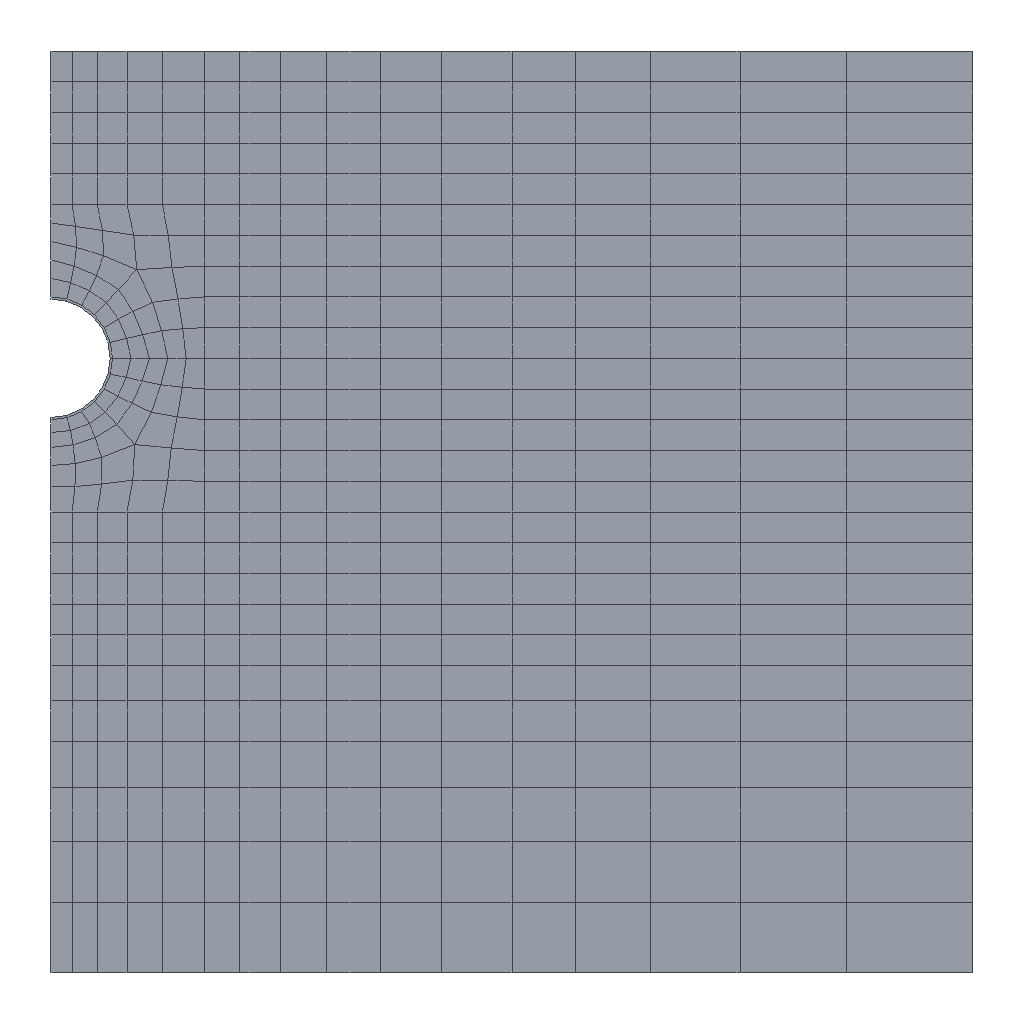Simulation study | abaqus
Set-up summary:
category,name,step,type,value,unit,region
solver,abaqus,,Abaqus/CAE 2024
units,mm-mN-s-kg (kPa) or mm-kg-s,,inferred,E=2e+07 density=
analysis,geo,,geostatic
analysis,relax-1,,static,time_period=1
analysis,add,,static,time_period=1
analysis,relax-2,,static,time_period=1
mesh,nodes,,,509
mesh,elements,,,446
element_type,CPE4,,,434
element_type,CPE4I,,,12
material,liner,,E,2e+07
material,liner,,nu,0.2
material,soil,,E,200000
material,soil,,nu,0.2
section,liner,,solid section,,,_PickedSet2
section,soil,,solid section,,,_PickedSet74
load,stress,initial,initial condition stress
load,Load-1,geo,by,-20,,_PickedSet6
load,,geo,concentrated force,"206.968 [dir=(0.9999, -0.0142, 0) n=2]",,soil-1.19
load,,geo,concentrated force,"273.813 [dir=(0.4268, -0.9043, 0) n=2]",,soil-1.20
load,,geo,concentrated force,"196.306 [dir=(0.5272, 0.8498, 0) n=2]",,soil-1.24
load,,geo,concentrated force,"239.406 [dir=(0.8773, -0.48, 0) n=2]",,soil-1.138
load,,geo,concentrated force,"301.488 [dir=(0.6514, -0.7587, 0) n=2]",,soil-1.139
load,,geo,concentrated force,"372.569 [dir=(0.445, -0.8955, 0) n=2]",,soil-1.140
load,,geo,concentrated force,"435.986 [dir=(0.2755, -0.9613, 0) n=2]",,soil-1.141
load,,geo,concentrated force,"479.559 [dir=(0.1318, -0.9913, 0) n=2]",,soil-1.142
load,,geo,concentrated force,"327.658 [dir=(0.1347, 0.9909, 0) n=2]",,soil-1.167
load,,geo,concentrated force,"310.398 [dir=(0.28, 0.96, 0) n=2]",,soil-1.168
load,,geo,concentrated force,"281.973 [dir=(0.4505, 0.8928, 0) n=2]",,soil-1.169
load,,geo,concentrated force,"246.244 [dir=(0.6591, 0.7521, 0) n=2]",,soil-1.170
load,,geo,concentrated force,"214.419 [dir=(0.8862, 0.4633, 0) n=2]",,soil-1.171
load,Load-2,relax-2,pressure,50,,_PickedSurf22
bc,BC-1,initial,fixed,[dofs=x],,_PickedSet12
bc,BC-2,initial,fixed,"[dofs=x,y n=2]",,_PickedSet13
bc,BC-3,initial,fixed,[dofs=x],,_PickedSet19
contact,Int-1,initial,contact pair surface to surface,interaction=IntProp-1; friction=0; behavior=hard,,tunnel / liner
Abaqus input file, long lists of numbers shortened:
*Heading
** Job name: deck Model name: Model-1
** Generated by: Abaqus/CAE 2024
*Preprint, echo=NO, model=NO, history=NO, contact=NO
**
** PARTS
**
*Part, name=Liner
*Node
      1,           0.,           4.
      2,           0.,    3.85
** (24 more lines like these left out)
*Element, type=CPE4I
 1,  1,  2,  4,  3
 2,  3,  4,  6,  5
** (10 more lines like these left out)
*Nset, nset=_PickedSet2, internal, generate
  1,  26,   1
*Elset, elset=_PickedSet2, internal, generate
  1,  12,   1
*Nset, nset=liner, generate
  1,  26,   1
*Elset, elset=liner, generate
  1,  12,   1
** Section: liner
*Solid Section, elset=_PickedSet2, material=liner
,
*End Part
**
*Part, name=soil
*Node
      1,          60.,         -10.
      2,          30.,         -10.
** (481 more lines like these left out)
*Element, type=CPE4
 1,   1,  27, 199,  42
 2,  27,  28, 200, 199
** (432 more lines like these left out)
*Nset, nset=all, generate
   1,  483,    1
*Elset, elset=all, generate
   1,  434,    1
*Nset, nset=_PickedSet74, internal, generate
   1,  483,    1
*Elset, elset=_PickedSet74, internal, generate
   1,  434,    1
*Nset, nset=tunnel
  19,  20,  24, 138, 139, 140, 141, 142, 167, 168, 169, 170, 171
*Elset, elset=tunnel
 214, 217, 220, 221, 222, 223, 292, 295, 298, 299, 300, 301
** Section: soil
*Solid Section, elset=_PickedSet74, material=soil
1.,
*End Part
**
**
** ASSEMBLY
**
*Assembly, name=Assembly
**
*Instance, name=soil-1, part=soil
*End Instance
**
*Instance, name=Liner-1, part=Liner
*End Instance
**
*Nset, nset=_PickedSet6, internal, instance=soil-1, generate
   1,  483,    1
*Elset, elset=_PickedSet6, internal, instance=soil-1, generate
   1,  434,    1
*Nset, nset=_PickedSet11, internal, instance=soil-1, generate
   1,  483,    1
*Elset, elset=_PickedSet11, internal, instance=soil-1, generate
   1,  434,    1
*Nset, nset=_PickedSet12, internal, instance=soil-1
   1,   4,   7,   8,  10,  11,  14,  20,  21,  22,  23,  24,  26,  39,  40,  41
  42,  52,  53,  54,  55,  56,  69,  70,  71,  72,  95,  96,  97,  98, 126, 127
** (2 more lines like these left out)
*Elset, elset=_PickedSet12, internal, instance=soil-1
   1,   6,  11,  16,  21,  50,  51,  52,  53,  54,  55,  76,  77,  78,  79,  80
 111, 116, 121, 126, 131, 196, 197, 223, 226, 229, 250, 251, 252, 253, 254, 259
** (2 more lines like these left out)
*Nset, nset=_PickedSet13, internal, instance=soil-1
   5,   8,  25,  26,  57,  58,  59,  60, 185, 186, 187, 188, 194, 195, 196, 197
 198,
*Elset, elset=_PickedSet13, internal, instance=soil-1
  26,  32,  38,  44,  50, 364, 365, 366, 367, 368, 404, 410, 416, 422, 428, 434
*Nset, nset=_PickedSet19, internal, instance=Liner-1
  1,  2, 25, 26
*Elset, elset=_PickedSet19, internal, instance=Liner-1
  1, 12
*Elset, elset=_liner_S4, internal, instance=Liner-1, generate
  1,  12,   1
*Surface, type=ELEMENT, name=liner
_liner_S4, S4
*Elset, elset=_tunnel_S2, internal, instance=soil-1
 214, 217, 220, 292, 295, 298
*Elset, elset=_tunnel_S1, internal, instance=soil-1
 221, 222, 223, 299, 300, 301
*Surface, type=ELEMENT, name=tunnel
_tunnel_S2, S2
_tunnel_S1, S1
*Elset, elset=__PickedSurf22_S4, internal, instance=soil-1, generate
 166,  191,    5
*Elset, elset=__PickedSurf22_S2, internal, instance=soil-1, generate
 234,  254,    5
*Surface, type=ELEMENT, name=_PickedSurf22, internal
__PickedSurf22_S4, S4
__PickedSurf22_S2, S2
*End Assembly
*Amplitude, name=Relax, time=TOTAL TIME
             0.,              1.,              1.,              1.,              2.,             0.6,              3.,             0.6
             4.,              0.
**
** MATERIALS
**
*Material, name=liner
*Elastic
 2e+07, 0.2
*Material, name=soil
*Elastic
200000., 0.2
**
** INTERACTION PROPERTIES
**
*Surface Interaction, name=IntProp-1
1.,
*Friction
0.,
*Surface Behavior, pressure-overclosure=HARD
**
** BOUNDARY CONDITIONS
**
** Name: BC-1 Type: Displacement/Rotation
*Boundary
_PickedSet12, 1, 1
** Name: BC-2 Type: Displacement/Rotation
*Boundary
_PickedSet13, 1, 1
_PickedSet13, 2, 2
** Name: BC-3 Type: Displacement/Rotation
*Boundary
_PickedSet19, 1, 1
**
** PREDEFINED FIELDS
**
** Name: stress   Type: Geostatic stress
*Initial Conditions, type=STRESS, GEOSTATIC
_PickedSet11, 0., 20., -1200., -40., 0.5, 0.5
**
** INTERACTIONS
**
** Interaction: Int-1
*Contact Pair, interaction=IntProp-1, type=SURFACE TO SURFACE
tunnel, liner
** ----------------------------------------------------------------
**
** STEP: geo
**
*Step, name=geo, nlgeom=NO
*Geostatic
**
** LOADS
**
** Name: Load-1   Type: Body force
*Dload
_PickedSet6, BY, -20.
*Cload,AMPLITUDE=RELAX
soil-1.19,1,206.947
soil-1.20,1,116.866
soil-1.24,1,103.483
soil-1.138,1,210.028
soil-1.139,1,196.399
soil-1.140,1,165.796
soil-1.141,1,120.131
soil-1.142,1,63.229
soil-1.167,1,44.15
soil-1.168,1,86.896
soil-1.169,1,127.017
soil-1.170,1,162.287
soil-1.171,1,190.018
soil-1.19,2,-2.939
soil-1.20,2,-247.62
soil-1.24,2,166.815
soil-1.138,2,-114.907
soil-1.139,2,-228.741
soil-1.140,2,-333.645
soil-1.141,2,-419.109
soil-1.142,2,-475.372
soil-1.167,2,324.67
soil-1.168,2,297.986
soil-1.169,2,251.745
soil-1.170,2,185.2
soil-1.171,2,99.341
**
** INTERACTIONS
**
** Interaction: Int-1
*Model Change, type=CONTACT PAIR, remove
tunnel, liner
** Interaction: Int-2
*Model Change, remove
Liner-1.liner,
**
** OUTPUT REQUESTS
**
*Restart, write, frequency=0
*Print, solve=NO
**
** FIELD OUTPUT: F-Output-1
**
*Output, field, variable=PRESELECT
**
** HISTORY OUTPUT: H-Output-1
**
*Output, history, variable=PRESELECT
*End Step
** ----------------------------------------------------------------
**
** STEP: relax-1
**
*Step, name=relax-1, nlgeom=NO
*Static
1., 1., 1e-05, 1.
**
** OUTPUT REQUESTS
**
*Restart, write, frequency=0
*Print, solve=YES
**
** FIELD OUTPUT: F-Output-1
**
*Output, field, variable=PRESELECT
**
** HISTORY OUTPUT: H-Output-1
**
*Output, history, variable=PRESELECT
*End Step
** ----------------------------------------------------------------
**
** STEP: add
**
*Step, name=add, nlgeom=NO
*Static
1., 1., 1e-05, 1.
**
** INTERACTIONS
**
** Interaction: Int-1
*Model Change, type=CONTACT PAIR, add
tunnel, liner
** Interaction: Int-2
*Model Change, add
Liner-1.liner,
**
** OUTPUT REQUESTS
**
*Restart, write, frequency=0
**
** FIELD OUTPUT: F-Output-1
**
*Output, field, variable=PRESELECT
**
** HISTORY OUTPUT: H-Output-1
**
*Output, history, variable=PRESELECT
*End Step
** ----------------------------------------------------------------
**
** STEP: relax-2
**
*Step, name=relax-2, nlgeom=NO
*Static
1., 1., 1e-05, 1.
**
** LOADS
**
** Name: Load-2   Type: Pressure
*Dsload
_PickedSurf22, P, 50.
**
** OUTPUT REQUESTS
**
*Restart, write, frequency=0
**
** FIELD OUTPUT: F-Output-1
**
*Output, field, variable=PRESELECT
**
** HISTORY OUTPUT: H-Output-1
**
*Output, history, variable=PRESELECT
*End Step
Results summary:
result,odb.job_status,,,JOB_STATUS_COMPLETED_SUCCESSFULLY,"consistent, unstated (Abaqus has no unit system)"
result,steps[0].procedure,geo,,*GEOSTATIC,"consistent, unstated (Abaqus has no unit system)"
result,steps[0].time_period,geo,,1,"consistent, unstated (Abaqus has no unit system)"
result,steps[0].n_frames,geo,,2,"consistent, unstated (Abaqus has no unit system)"
result,steps[0].last_frame.id,geo,,1,"consistent, unstated (Abaqus has no unit system)"
result,steps[0].last_frame.value,geo,,1,"consistent, unstated (Abaqus has no unit system)"
result,steps[0].last_frame.description,geo,,Increment      1: Step Time =    1.000,"consistent, unstated (Abaqus has no unit system)"
result,steps[0].completed,geo,,True,"consistent, unstated (Abaqus has no unit system)"
result,steps[0].max_U_magnitude,geo,,2.12286e-05,"consistent, unstated (Abaqus has no unit system)"
result,steps[0].max_S_mises,geo,,577.079,"consistent, unstated (Abaqus has no unit system)"
result,steps[0].RF_sum[1],geo,,-1793.25,"consistent, unstated (Abaqus has no unit system)"
result,steps[0].RF_sum[2],geo,,71999.6,"consistent, unstated (Abaqus has no unit system)"
result,steps[1].procedure,relax-1,,*STATIC,"consistent, unstated (Abaqus has no unit system)"
result,steps[1].time_period,relax-1,,1,"consistent, unstated (Abaqus has no unit system)"
result,steps[1].n_frames,relax-1,,2,"consistent, unstated (Abaqus has no unit system)"
result,steps[1].last_frame.id,relax-1,,1,"consistent, unstated (Abaqus has no unit system)"
result,steps[1].last_frame.value,relax-1,,1,"consistent, unstated (Abaqus has no unit system)"
result,steps[1].last_frame.description,relax-1,,Increment      1: Step Time =    1.000,"consistent, unstated (Abaqus has no unit system)"
result,steps[1].completed,relax-1,,True,"consistent, unstated (Abaqus has no unit system)"
result,steps[1].max_U_magnitude,relax-1,,0.00595,"consistent, unstated (Abaqus has no unit system)"
result,steps[1].max_S_mises,relax-1,,576.778,"consistent, unstated (Abaqus has no unit system)"
result,steps[1].RF_sum[1],relax-1,,-1075.95,"consistent, unstated (Abaqus has no unit system)"
result,steps[1].RF_sum[2],relax-1,,71801,"consistent, unstated (Abaqus has no unit system)"
result,steps[2].procedure,add,,*STATIC,"consistent, unstated (Abaqus has no unit system)"
result,steps[2].time_period,add,,1,"consistent, unstated (Abaqus has no unit system)"
result,steps[2].n_frames,add,,2,"consistent, unstated (Abaqus has no unit system)"
result,steps[2].last_frame.id,add,,1,"consistent, unstated (Abaqus has no unit system)"
result,steps[2].last_frame.value,add,,1,"consistent, unstated (Abaqus has no unit system)"
result,steps[2].last_frame.description,add,,Increment      1: Step Time =    1.000,"consistent, unstated (Abaqus has no unit system)"
result,steps[2].completed,add,,True,"consistent, unstated (Abaqus has no unit system)"
result,steps[2].max_U_magnitude,add,,0.004011,"consistent, unstated (Abaqus has no unit system)"
result,steps[2].max_S_mises,add,,2724.15,"consistent, unstated (Abaqus has no unit system)"
result,steps[2].RF_sum[1],add,,-1075.95,"consistent, unstated (Abaqus has no unit system)"
result,steps[2].RF_sum[2],add,,71801,"consistent, unstated (Abaqus has no unit system)"
result,steps[3].procedure,relax-2,,*STATIC,"consistent, unstated (Abaqus has no unit system)"
result,steps[3].time_period,relax-2,,1,"consistent, unstated (Abaqus has no unit system)"
result,steps[3].n_frames,relax-2,,2,"consistent, unstated (Abaqus has no unit system)"
result,steps[3].last_frame.id,relax-2,,1,"consistent, unstated (Abaqus has no unit system)"
result,steps[3].last_frame.value,relax-2,,1,"consistent, unstated (Abaqus has no unit system)"
result,steps[3].last_frame.description,relax-2,,Increment      1: Step Time =    1.000,"consistent, unstated (Abaqus has no unit system)"
result,steps[3].completed,relax-2,,True,"consistent, unstated (Abaqus has no unit system)"
result,steps[3].max_U_magnitude,relax-2,,0.0126,"consistent, unstated (Abaqus has no unit system)"
result,steps[3].max_S_mises,relax-2,,7915.84,"consistent, unstated (Abaqus has no unit system)"
result,steps[3].RF_sum[1],relax-2,,-0.03214,"consistent, unstated (Abaqus has no unit system)"
result,steps[3].RF_sum[2],relax-2,,73003.1,"consistent, unstated (Abaqus has no unit system)"